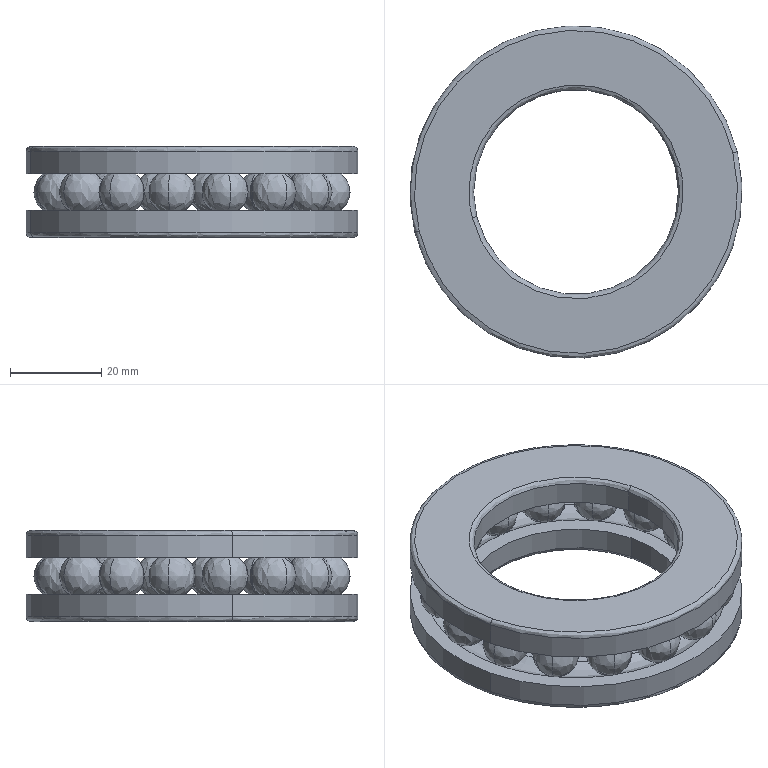Part | SolidWorks | features BaseBody 1 | 1 solid | 86 faces | box 73 x 73 x 20 mm | volume 37195 mm3 | spline 72 | cylinder 8 | plane 6 | commonest cylinder face diameters 73 x4 45 x2 47 x2